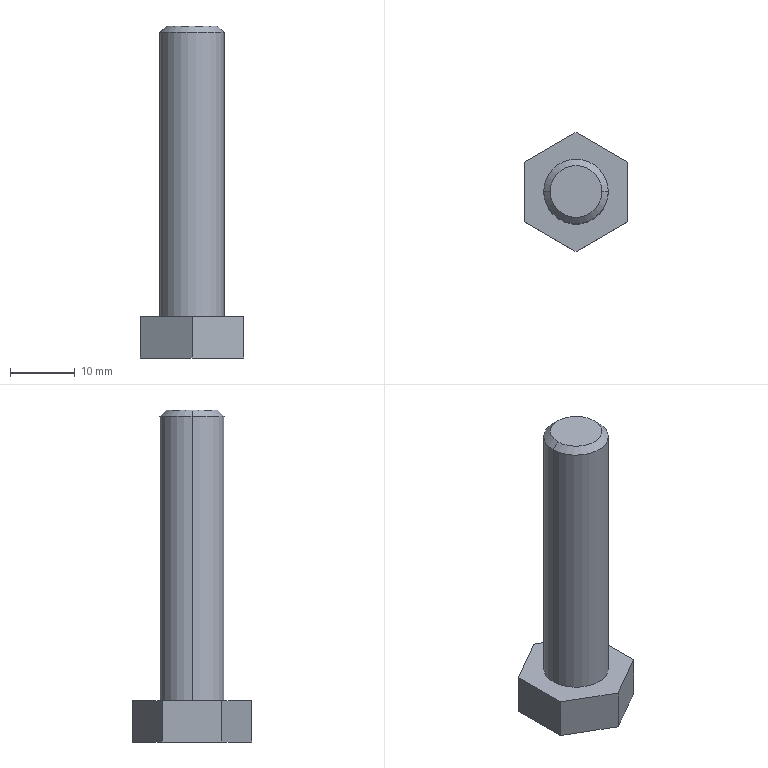Part | SolidWorks | features Chamfer 1, Extrusion 1, ICE 1, RefAxis 1 | 1 solid | 13 faces | box 16 x 18.475 x 51.4 mm | volume 4939 mm3 | plane 9 | cone 2 | cylinder 2 | commonest cylinder face diameters 10 x2
STEP:
#1=CARTESIAN_POINT('',(4.,0.,51.4));
#2=VERTEX_POINT('',#1);
#3=CARTESIAN_POINT('',(-4.,0.,51.4));
#4=VERTEX_POINT('',#3);
#5=CARTESIAN_POINT('',(0.,0.,51.4));
#6=DIRECTION('',(0.,0.,1.));
#7=DIRECTION('',(1.,0.,0.));
#8=AXIS2_PLACEMENT_3D('',#5,#6,#7);
#9=CIRCLE('',#8,4.);
#10=EDGE_CURVE('',#2,#4,#9,.T.);
#11=ORIENTED_EDGE('',*,*,#10,.F.);
#12=CARTESIAN_POINT('',(5.,0.,50.4));
#13=VERTEX_POINT('',#12);
#14=CARTESIAN_POINT('',(4.,0.,51.4));
#15=DIRECTION('',(0.7071,0.,-0.7071));
#16=VECTOR('',#15,1000.);
#17=LINE('',#14,#16);
#18=EDGE_CURVE('',#2,#13,#17,.T.);
#19=ORIENTED_EDGE('',*,*,#18,.T.);
#20=CARTESIAN_POINT('',(-5.,0.,50.4));
#21=VERTEX_POINT('',#20);
#22=CARTESIAN_POINT('',(0.,0.,50.4));
#23=DIRECTION('',(0.,0.,-1.));
#24=DIRECTION('',(1.,0.,0.));
#25=AXIS2_PLACEMENT_3D('',#22,#23,#24);
#26=CIRCLE('',#25,5.);
#27=EDGE_CURVE('',#21,#13,#26,.T.);
#28=ORIENTED_EDGE('',*,*,#27,.F.);
#29=CARTESIAN_POINT('',(-4.,0.,51.4));
#30=DIRECTION('',(-0.7071,0.,-0.7071));
#31=VECTOR('',#30,1000.);
#32=LINE('',#29,#31);
#33=EDGE_CURVE('',#4,#21,#32,.T.);
#34=ORIENTED_EDGE('',*,*,#33,.F.);
#35=EDGE_LOOP('',(#11,#19,#28,#34));
#36=FACE_OUTER_BOUND('',#35,.T.);
#37=CARTESIAN_POINT('',(0.,0.,51.4));
#38=DIRECTION('',(0.,0.,-1.));
#39=DIRECTION('',(-1.,0.,0.));
#40=AXIS2_PLACEMENT_3D('',#37,#38,#39);
#41=CONICAL_SURFACE('',#40,4.,0.7854);
#42=ADVANCED_FACE('',(#36),#41,.T.);
#43=ORIENTED_EDGE('',*,*,#27,.T.);
#44=CARTESIAN_POINT('',(5.,0.,6.4));
#45=VERTEX_POINT('',#44);
#46=CARTESIAN_POINT('',(5.,0.,51.4));
#47=DIRECTION('',(0.,0.,-1.));
#48=VECTOR('',#47,1000.);
#49=LINE('',#46,#48);
#50=EDGE_CURVE('',#13,#45,#49,.T.);
#51=ORIENTED_EDGE('',*,*,#50,.T.);
#52=CARTESIAN_POINT('',(-5.,0.,6.4));
#53=VERTEX_POINT('',#52);
#54=CARTESIAN_POINT('',(0.,0.,6.4));
#55=DIRECTION('',(0.,0.,1.));
#56=DIRECTION('',(1.,0.,0.));
#57=AXIS2_PLACEMENT_3D('',#54,#55,#56);
#58=CIRCLE('',#57,5.);
#59=EDGE_CURVE('',#45,#53,#58,.T.);
#60=ORIENTED_EDGE('',*,*,#59,.T.);
#61=CARTESIAN_POINT('',(-5.,0.,51.4));
#62=DIRECTION('',(0.,0.,-1.));
#63=VECTOR('',#62,1000.);
#64=LINE('',#61,#63);
#65=EDGE_CURVE('',#21,#53,#64,.T.);
#66=ORIENTED_EDGE('',*,*,#65,.F.);
#67=EDGE_LOOP('',(#43,#51,#60,#66));
#68=FACE_OUTER_BOUND('',#67,.T.);
#69=CARTESIAN_POINT('',(0.,0.,51.4));
#70=DIRECTION('',(0.,0.,-1.));
#71=DIRECTION('',(-1.,0.,0.));
#72=AXIS2_PLACEMENT_3D('',#69,#70,#71);
#73=CYLINDRICAL_SURFACE('',#72,5.);
#74=ADVANCED_FACE('',(#68),#73,.T.);
#75=CARTESIAN_POINT('',(8.,-4.619,6.4));
#76=VERTEX_POINT('',#75);
#77=CARTESIAN_POINT('',(8.,4.619,6.4));
#78=VERTEX_POINT('',#77);
#79=CARTESIAN_POINT('',(8.,-4.619,6.4));
#80=DIRECTION('',(0.,1.,0.));
#81=VECTOR('',#80,1000.);
#82=LINE('',#79,#81);
#83=EDGE_CURVE('',#76,#78,#82,.T.);
#84=ORIENTED_EDGE('',*,*,#83,.T.);
#85=CARTESIAN_POINT('',(0.,9.238,6.4));
#86=VERTEX_POINT('',#85);
#87=CARTESIAN_POINT('',(8.,4.619,6.4));
#88=DIRECTION('',(-0.866,0.5,0.));
#89=VECTOR('',#88,1000.);
#90=LINE('',#87,#89);
#91=EDGE_CURVE('',#78,#86,#90,.T.);
#92=ORIENTED_EDGE('',*,*,#91,.T.);
#93=CARTESIAN_POINT('',(-8.,4.619,6.4));
#94=VERTEX_POINT('',#93);
#95=CARTESIAN_POINT('',(0.,9.238,6.4));
#96=DIRECTION('',(-0.866,-0.5,0.));
#97=VECTOR('',#96,1000.);
#98=LINE('',#95,#97);
#99=EDGE_CURVE('',#86,#94,#98,.T.);
#100=ORIENTED_EDGE('',*,*,#99,.T.);
#101=CARTESIAN_POINT('',(-8.,-4.619,6.4));
#102=VERTEX_POINT('',#101);
#103=CARTESIAN_POINT('',(-8.,4.619,6.4));
#104=DIRECTION('',(0.,-1.,0.));
#105=VECTOR('',#104,1000.);
#106=LINE('',#103,#105);
#107=EDGE_CURVE('',#94,#102,#106,.T.);
#108=ORIENTED_EDGE('',*,*,#107,.T.);
#109=CARTESIAN_POINT('',(0.,-9.238,6.4));
#110=VERTEX_POINT('',#109);
#111=CARTESIAN_POINT('',(-8.,-4.619,6.4));
#112=DIRECTION('',(0.866,-0.5,0.));
#113=VECTOR('',#112,1000.);
#114=LINE('',#111,#113);
#115=EDGE_CURVE('',#102,#110,#114,.T.);
#116=ORIENTED_EDGE('',*,*,#115,.T.);
#117=CARTESIAN_POINT('',(0.,-9.238,6.4));
#118=DIRECTION('',(0.866,0.5,0.));
#119=VECTOR('',#118,1000.);
#120=LINE('',#117,#119);
#121=EDGE_CURVE('',#110,#76,#120,.T.);
#122=ORIENTED_EDGE('',*,*,#121,.T.);
#123=EDGE_LOOP('',(#84,#92,#100,#108,#116,#122));
#124=FACE_OUTER_BOUND('',#123,.T.);
#125=CARTESIAN_POINT('',(0.,0.,6.4));
#126=DIRECTION('',(0.,0.,1.));
#127=DIRECTION('',(1.,0.,0.));
#128=AXIS2_PLACEMENT_3D('',#125,#126,#127);
#129=CIRCLE('',#128,5.);
#130=EDGE_CURVE('',#53,#45,#129,.T.);
#131=ORIENTED_EDGE('',*,*,#130,.F.);
#132=ORIENTED_EDGE('',*,*,#59,.F.);
#133=EDGE_LOOP('',(#131,#132));
#134=FACE_BOUND('',#133,.T.);
#135=CARTESIAN_POINT('',(0.,0.,6.4));
#136=DIRECTION('',(0.,0.,1.));
#137=DIRECTION('',(1.,0.,0.));
#138=AXIS2_PLACEMENT_3D('',#135,#136,#137);
#139=PLANE('',#138);
#140=ADVANCED_FACE('',(#124,#134),#139,.T.);
#141=CARTESIAN_POINT('',(8.,-4.619,0.));
#142=VERTEX_POINT('',#141);
#143=CARTESIAN_POINT('',(8.,4.619,0.));
#144=VERTEX_POINT('',#143);
#145=CARTESIAN_POINT('',(8.,-4.619,0.));
#146=DIRECTION('',(0.,1.,0.));
#147=VECTOR('',#146,1000.);
#148=LINE('',#145,#147);
#149=EDGE_CURVE('',#142,#144,#148,.T.);
#150=ORIENTED_EDGE('',*,*,#149,.T.);
#151=CARTESIAN_POINT('',(8.,4.619,6.4));
#152=DIRECTION('',(0.,0.,-1.));
#153=VECTOR('',#152,1000.);
#154=LINE('',#151,#153);
#155=EDGE_CURVE('',#78,#144,#154,.T.);
#156=ORIENTED_EDGE('',*,*,#155,.F.);
#157=ORIENTED_EDGE('',*,*,#83,.F.);
#158=CARTESIAN_POINT('',(8.,-4.619,6.4));
#159=DIRECTION('',(0.,0.,-1.));
#160=VECTOR('',#159,1000.);
#161=LINE('',#158,#160);
#162=EDGE_CURVE('',#76,#142,#161,.T.);
#163=ORIENTED_EDGE('',*,*,#162,.T.);
#164=EDGE_LOOP('',(#150,#156,#157,#163));
#165=FACE_OUTER_BOUND('',#164,.T.);
#166=CARTESIAN_POINT('',(8.,-4.619,6.4));
#167=DIRECTION('',(-1.,0.,0.));
#168=DIRECTION('',(0.,-1.,0.));
#169=AXIS2_PLACEMENT_3D('',#166,#167,#168);
#170=PLANE('',#169);
#171=ADVANCED_FACE('',(#165),#170,.F.);
#172=CARTESIAN_POINT('',(0.,9.238,0.));
#173=VERTEX_POINT('',#172);
#174=CARTESIAN_POINT('',(8.,4.619,0.));
#175=DIRECTION('',(-0.866,0.5,0.));
#176=VECTOR('',#175,1000.);
#177=LINE('',#174,#176);
#178=EDGE_CURVE('',#144,#173,#177,.T.);
#179=ORIENTED_EDGE('',*,*,#178,.T.);
#180=CARTESIAN_POINT('',(0.,9.238,6.4));
#181=DIRECTION('',(0.,0.,-1.));
#182=VECTOR('',#181,1000.);
#183=LINE('',#180,#182);
#184=EDGE_CURVE('',#86,#173,#183,.T.);
#185=ORIENTED_EDGE('',*,*,#184,.F.);
#186=ORIENTED_EDGE('',*,*,#91,.F.);
#187=ORIENTED_EDGE('',*,*,#155,.T.);
#188=EDGE_LOOP('',(#179,#185,#186,#187));
#189=FACE_OUTER_BOUND('',#188,.T.);
#190=CARTESIAN_POINT('',(8.,4.619,6.4));
#191=DIRECTION('',(-0.5,-0.866,0.));
#192=DIRECTION('',(0.866,-0.5,0.));
#193=AXIS2_PLACEMENT_3D('',#190,#191,#192);
#194=PLANE('',#193);
#195=ADVANCED_FACE('',(#189),#194,.F.);
#196=CARTESIAN_POINT('',(-8.,4.619,0.));
#197=VERTEX_POINT('',#196);
#198=CARTESIAN_POINT('',(0.,9.238,0.));
#199=DIRECTION('',(-0.866,-0.5,0.));
#200=VECTOR('',#199,1000.);
#201=LINE('',#198,#200);
#202=EDGE_CURVE('',#173,#197,#201,.T.);
#203=ORIENTED_EDGE('',*,*,#202,.T.);
#204=CARTESIAN_POINT('',(-8.,4.619,6.4));
#205=DIRECTION('',(0.,0.,-1.));
#206=VECTOR('',#205,1000.);
#207=LINE('',#204,#206);
#208=EDGE_CURVE('',#94,#197,#207,.T.);
#209=ORIENTED_EDGE('',*,*,#208,.F.);
#210=ORIENTED_EDGE('',*,*,#99,.F.);
#211=ORIENTED_EDGE('',*,*,#184,.T.);
#212=EDGE_LOOP('',(#203,#209,#210,#211));
#213=FACE_OUTER_BOUND('',#212,.T.);
#214=CARTESIAN_POINT('',(0.,9.238,6.4));
#215=DIRECTION('',(0.5,-0.866,0.));
#216=DIRECTION('',(0.866,0.5,0.));
#217=AXIS2_PLACEMENT_3D('',#214,#215,#216);
#218=PLANE('',#217);
#219=ADVANCED_FACE('',(#213),#218,.F.);
#220=CARTESIAN_POINT('',(-8.,-4.619,0.));
#221=VERTEX_POINT('',#220);
#222=CARTESIAN_POINT('',(-8.,4.619,0.));
#223=DIRECTION('',(0.,-1.,0.));
#224=VECTOR('',#223,1000.);
#225=LINE('',#222,#224);
#226=EDGE_CURVE('',#197,#221,#225,.T.);
#227=ORIENTED_EDGE('',*,*,#226,.T.);
#228=CARTESIAN_POINT('',(-8.,-4.619,6.4));
#229=DIRECTION('',(0.,0.,-1.));
#230=VECTOR('',#229,1000.);
#231=LINE('',#228,#230);
#232=EDGE_CURVE('',#102,#221,#231,.T.);
#233=ORIENTED_EDGE('',*,*,#232,.F.);
#234=ORIENTED_EDGE('',*,*,#107,.F.);
#235=ORIENTED_EDGE('',*,*,#208,.T.);
#236=EDGE_LOOP('',(#227,#233,#234,#235));
#237=FACE_OUTER_BOUND('',#236,.T.);
#238=CARTESIAN_POINT('',(-8.,4.619,6.4));
#239=DIRECTION('',(1.,0.,0.));
#240=DIRECTION('',(0.,1.,0.));
#241=AXIS2_PLACEMENT_3D('',#238,#239,#240);
#242=PLANE('',#241);
#243=ADVANCED_FACE('',(#237),#242,.F.);
#244=CARTESIAN_POINT('',(0.,-9.238,0.));
#245=VERTEX_POINT('',#244);
#246=CARTESIAN_POINT('',(-8.,-4.619,0.));
#247=DIRECTION('',(0.866,-0.5,0.));
#248=VECTOR('',#247,1000.);
#249=LINE('',#246,#248);
#250=EDGE_CURVE('',#221,#245,#249,.T.);
#251=ORIENTED_EDGE('',*,*,#250,.T.);
#252=CARTESIAN_POINT('',(0.,-9.238,6.4));
#253=DIRECTION('',(0.,0.,-1.));
#254=VECTOR('',#253,1000.);
#255=LINE('',#252,#254);
#256=EDGE_CURVE('',#110,#245,#255,.T.);
#257=ORIENTED_EDGE('',*,*,#256,.F.);
#258=ORIENTED_EDGE('',*,*,#115,.F.);
#259=ORIENTED_EDGE('',*,*,#232,.T.);
#260=EDGE_LOOP('',(#251,#257,#258,#259));
#261=FACE_OUTER_BOUND('',#260,.T.);
#262=CARTESIAN_POINT('',(-8.,-4.619,6.4));
#263=DIRECTION('',(0.5,0.866,0.));
#264=DIRECTION('',(-0.866,0.5,0.));
#265=AXIS2_PLACEMENT_3D('',#262,#263,#264);
#266=PLANE('',#265);
#267=ADVANCED_FACE('',(#261),#266,.F.);
#268=CARTESIAN_POINT('',(0.,-9.238,0.));
#269=DIRECTION('',(0.866,0.5,0.));
#270=VECTOR('',#269,1000.);
#271=LINE('',#268,#270);
#272=EDGE_CURVE('',#245,#142,#271,.T.);
#273=ORIENTED_EDGE('',*,*,#272,.T.);
#274=ORIENTED_EDGE('',*,*,#162,.F.);
#275=ORIENTED_EDGE('',*,*,#121,.F.);
#276=ORIENTED_EDGE('',*,*,#256,.T.);
#277=EDGE_LOOP('',(#273,#274,#275,#276));
#278=FACE_OUTER_BOUND('',#277,.T.);
#279=CARTESIAN_POINT('',(0.,-9.238,6.4));
#280=DIRECTION('',(-0.5,0.866,0.));
#281=DIRECTION('',(-0.866,-0.5,0.));
#282=AXIS2_PLACEMENT_3D('',#279,#280,#281);
#283=PLANE('',#282);
#284=ADVANCED_FACE('',(#278),#283,.F.);
#285=ORIENTED_EDGE('',*,*,#149,.F.);
#286=ORIENTED_EDGE('',*,*,#272,.F.);
#287=ORIENTED_EDGE('',*,*,#250,.F.);
#288=ORIENTED_EDGE('',*,*,#226,.F.);
#289=ORIENTED_EDGE('',*,*,#202,.F.);
#290=ORIENTED_EDGE('',*,*,#178,.F.);
#291=EDGE_LOOP('',(#285,#286,#287,#288,#289,#290));
#292=FACE_OUTER_BOUND('',#291,.T.);
#293=CARTESIAN_POINT('',(0.,0.,0.));
#294=DIRECTION('',(0.,0.,1.));
#295=DIRECTION('',(1.,0.,0.));
#296=AXIS2_PLACEMENT_3D('',#293,#294,#295);
#297=PLANE('',#296);
#298=ADVANCED_FACE('',(#292),#297,.F.);
#299=ORIENTED_EDGE('',*,*,#50,.F.);
#300=CARTESIAN_POINT('',(0.,0.,50.4));
#301=DIRECTION('',(0.,0.,-1.));
#302=DIRECTION('',(1.,0.,0.));
#303=AXIS2_PLACEMENT_3D('',#300,#301,#302);
#304=CIRCLE('',#303,5.);
#305=EDGE_CURVE('',#13,#21,#304,.T.);
#306=ORIENTED_EDGE('',*,*,#305,.T.);
#307=ORIENTED_EDGE('',*,*,#65,.T.);
#308=ORIENTED_EDGE('',*,*,#130,.T.);
#309=EDGE_LOOP('',(#299,#306,#307,#308));
#310=FACE_OUTER_BOUND('',#309,.T.);
#311=CARTESIAN_POINT('',(0.,0.,51.4));
#312=DIRECTION('',(0.,0.,-1.));
#313=DIRECTION('',(-1.,0.,0.));
#314=AXIS2_PLACEMENT_3D('',#311,#312,#313);
#315=CYLINDRICAL_SURFACE('',#314,5.);
#316=ADVANCED_FACE('',(#310),#315,.T.);
#317=CARTESIAN_POINT('',(0.,0.,51.4));
#318=DIRECTION('',(0.,0.,1.));
#319=DIRECTION('',(1.,0.,0.));
#320=AXIS2_PLACEMENT_3D('',#317,#318,#319);
#321=CIRCLE('',#320,4.);
#322=EDGE_CURVE('',#4,#2,#321,.T.);
#323=ORIENTED_EDGE('',*,*,#322,.T.);
#324=ORIENTED_EDGE('',*,*,#10,.T.);
#325=EDGE_LOOP('',(#323,#324));
#326=FACE_OUTER_BOUND('',#325,.T.);
#327=CARTESIAN_POINT('',(0.,0.,51.4));
#328=DIRECTION('',(0.,0.,1.));
#329=DIRECTION('',(1.,0.,0.));
#330=AXIS2_PLACEMENT_3D('',#327,#328,#329);
#331=PLANE('',#330);
#332=ADVANCED_FACE('',(#326),#331,.T.);
#333=ORIENTED_EDGE('',*,*,#18,.F.);
#334=ORIENTED_EDGE('',*,*,#322,.F.);
#335=ORIENTED_EDGE('',*,*,#33,.T.);
#336=ORIENTED_EDGE('',*,*,#305,.F.);
#337=EDGE_LOOP('',(#333,#334,#335,#336));
#338=FACE_OUTER_BOUND('',#337,.T.);
#339=CARTESIAN_POINT('',(0.,0.,51.4));
#340=DIRECTION('',(0.,0.,-1.));
#341=DIRECTION('',(-1.,0.,0.));
#342=AXIS2_PLACEMENT_3D('',#339,#340,#341);
#343=CONICAL_SURFACE('',#342,4.,0.7854);
#344=ADVANCED_FACE('',(#338),#343,.T.);
#345=CLOSED_SHELL('',(#42,#74,#140,#171,#195,#219,#243,#267,#284,#298,#316,#332,#344));
#346=MANIFOLD_SOLID_BREP('',#345);
#347=CARTESIAN_POINT('',(0.,0.,0.));
#348=DIRECTION('',(0.,0.,1.));
#349=DIRECTION('',(1.,0.,0.));
#350=AXIS2_PLACEMENT_3D('',#347,#348,#349);
#351=(LENGTH_UNIT()NAMED_UNIT(*)SI_UNIT(.MILLI.,.METRE.));
#352=UNCERTAINTY_MEASURE_WITH_UNIT(LENGTH_MEASURE(0.00001),#351,'','');
#353=(NAMED_UNIT(*)PLANE_ANGLE_UNIT()SI_UNIT($,.RADIAN.));
#354=(NAMED_UNIT(*)SI_UNIT($,.STERADIAN.)SOLID_ANGLE_UNIT());
#355=(GEOMETRIC_REPRESENTATION_CONTEXT(3)GLOBAL_UNCERTAINTY_ASSIGNED_CONTEXT((#352))GLOBAL_UNIT_ASSIGNED_CONTEXT((#351,#353,#354))REPRESENTATION_CONTEXT('',''));
#356=ADVANCED_BREP_SHAPE_REPRESENTATION('',(#346,#350),#355);